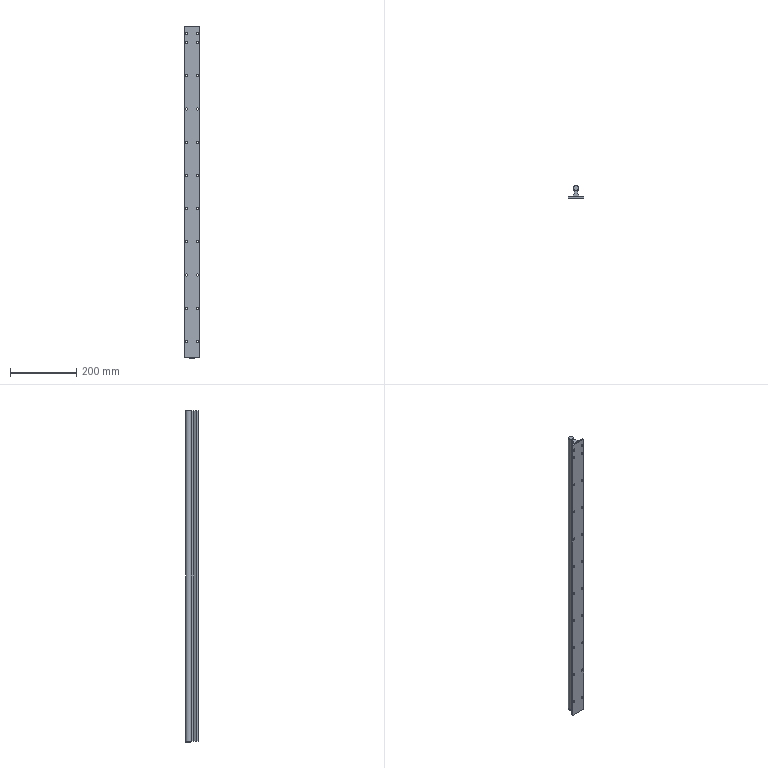Part | STEP file | b7-ashw-16-1000 | 1 solid | 64 faces | box 48 x 38 x 1000 mm | volume 648601 mm3 | cylinder 44 | plane 16 | cone 4 | commonest cylinder face diameters 7 x42 16 x2